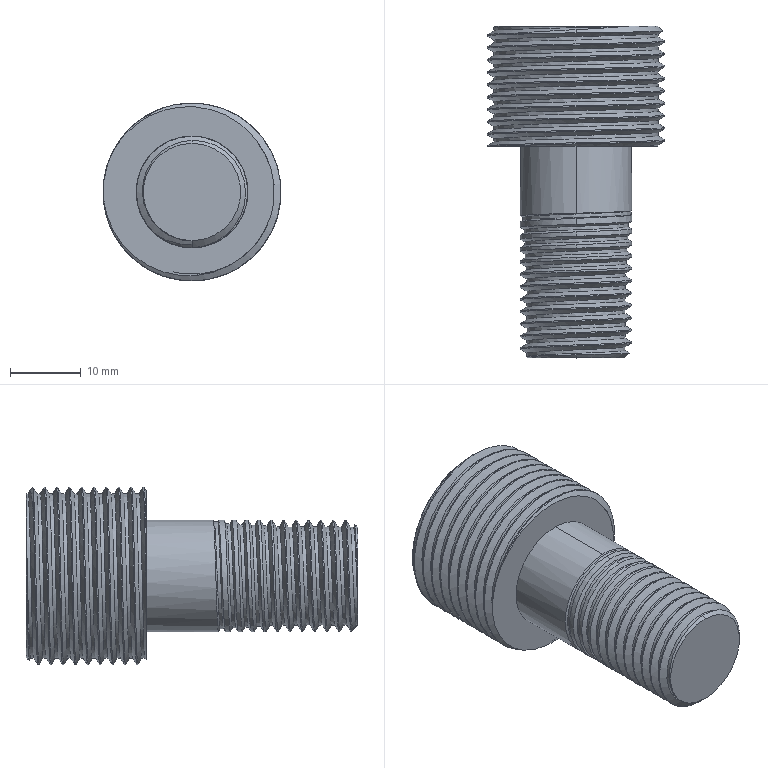Part | SolidWorks | features Helix 2, SweepCut 2, Revolution 1 | 1 solid | 58 faces | box 25.2 x 47 x 25.2 mm | volume 13171 mm3 | cylinder 42 | cone 6 | spline 6 | plane 4 | commonest cylinder face diameters 15.8 x23 25.2 x19